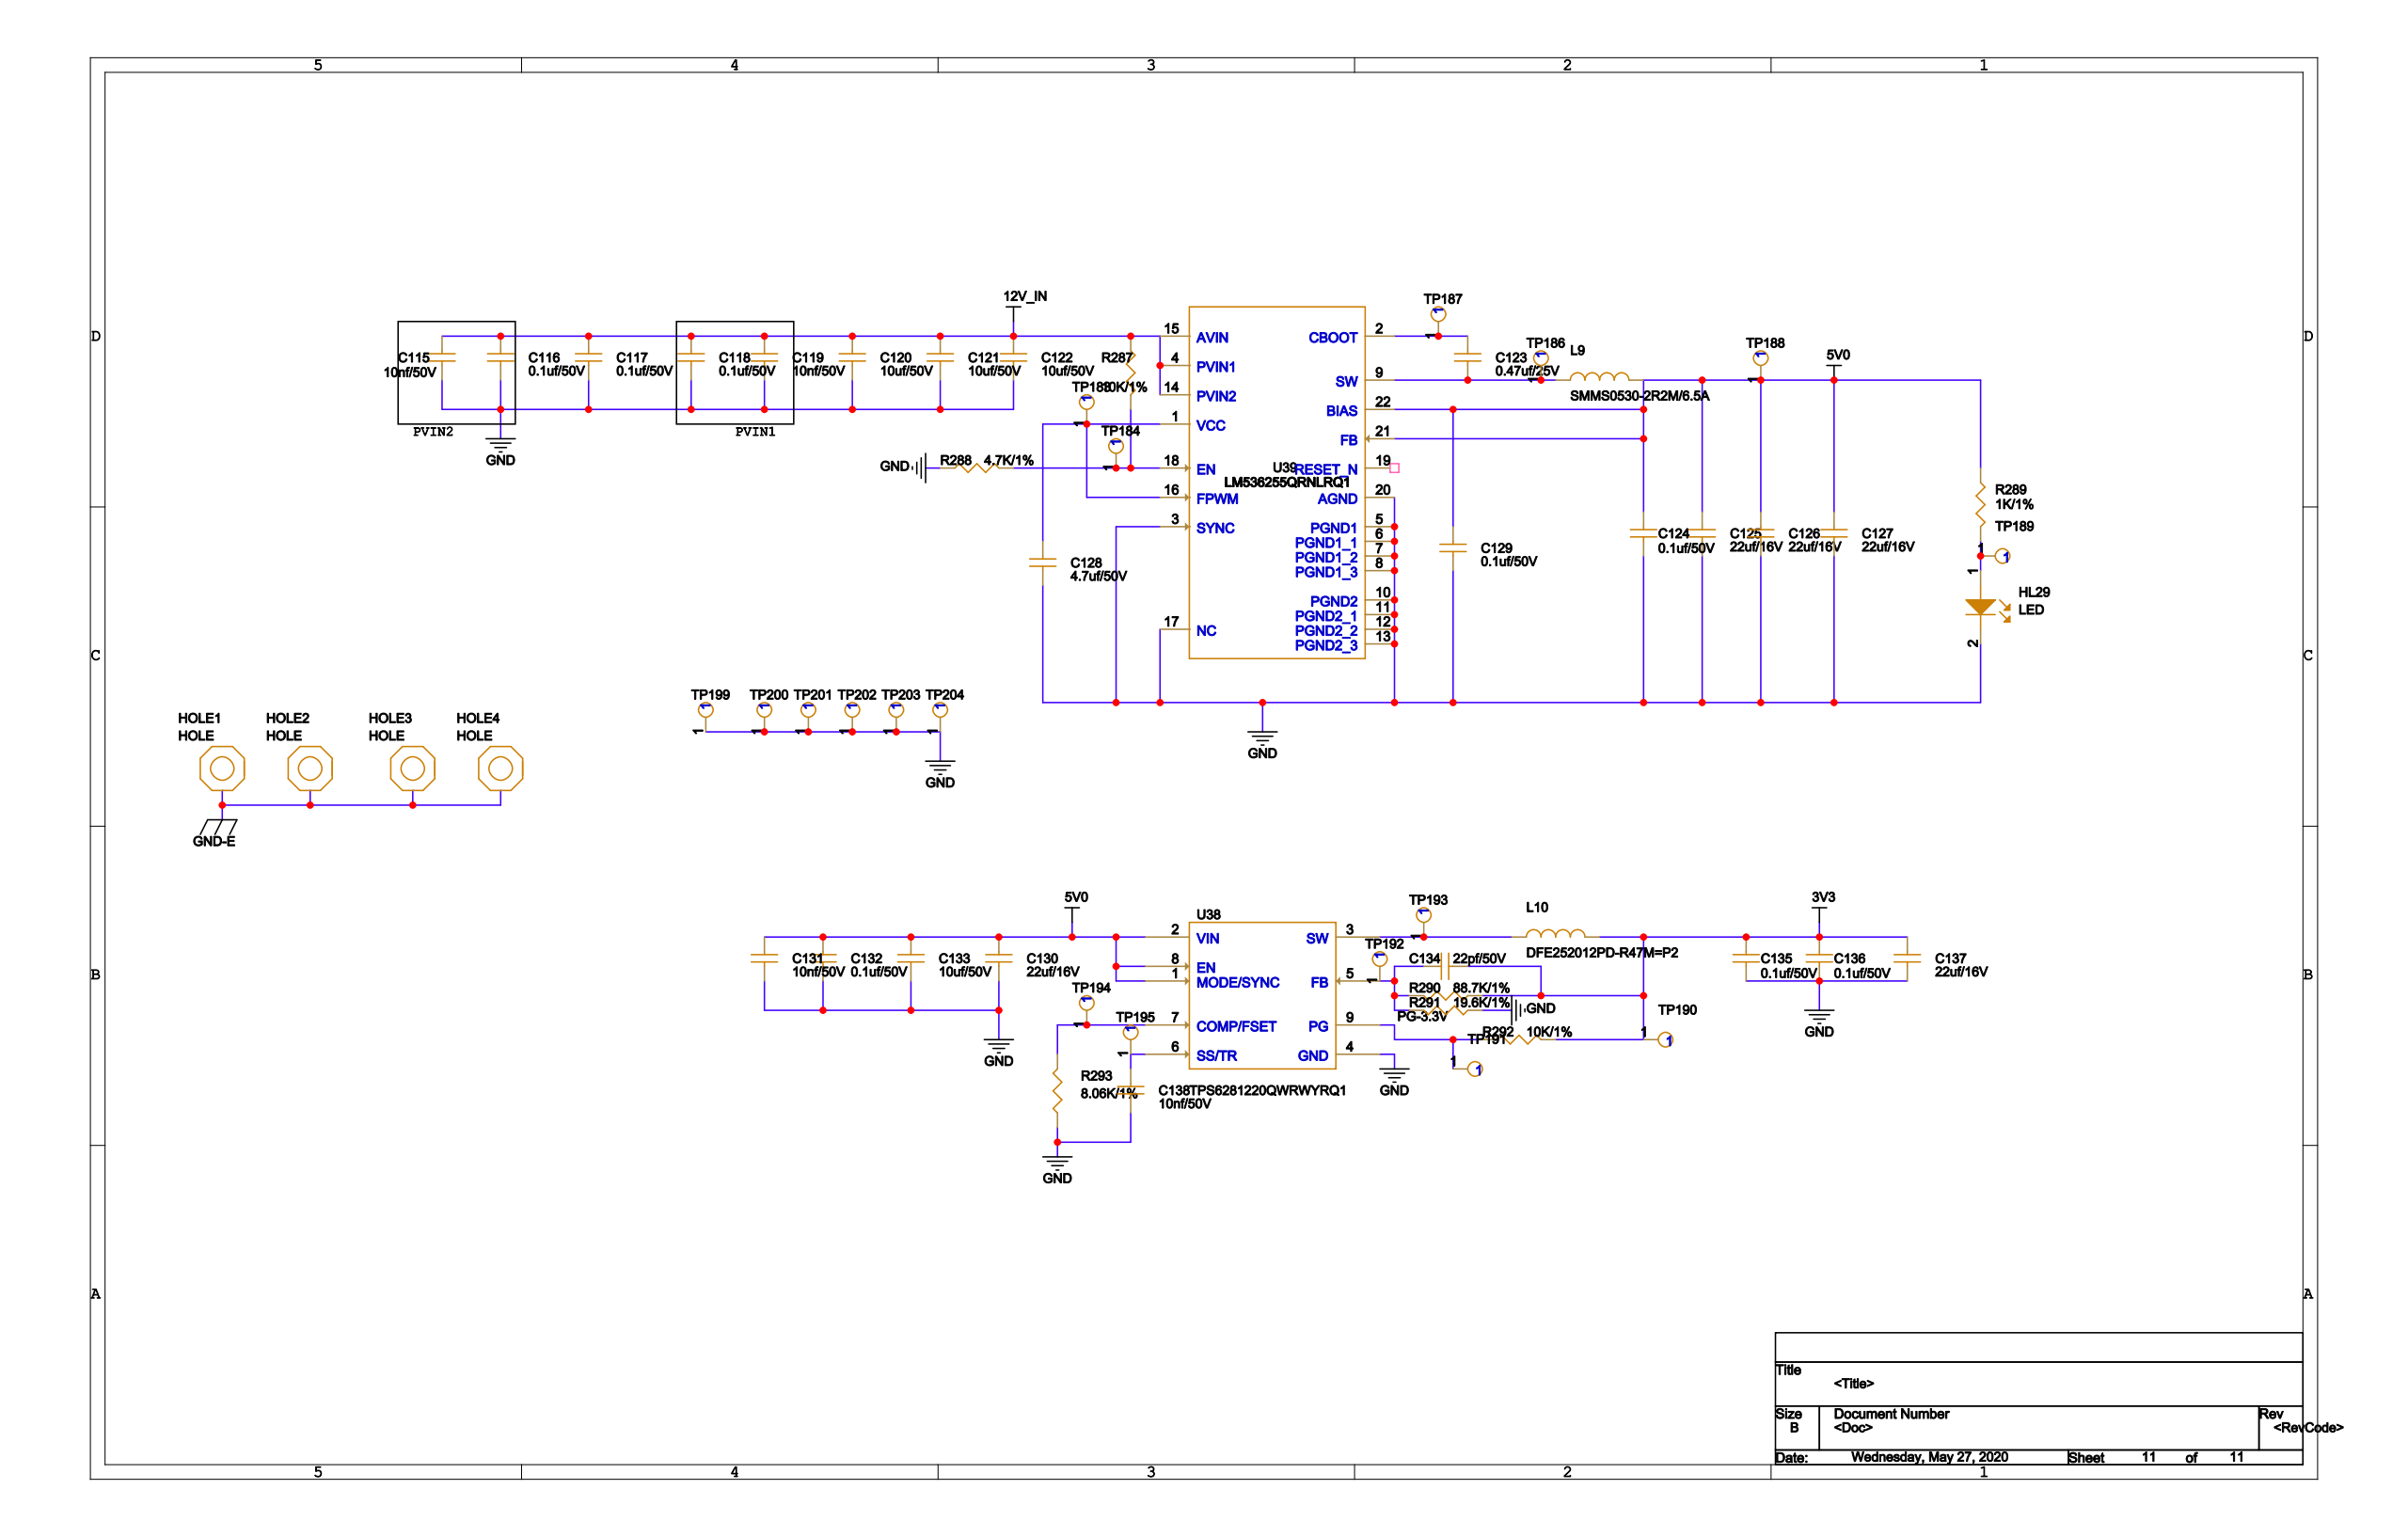Circuit board | Cadence Allegro | 521 parts | 239 nets | one sheet of the schematic
Parts on this sheet (reference | value | footprint):
C115 | 10nf/50V | C0402
C116 | 0.1uf/50V | C0402
C117 | 0.1uf/50V | C0402
C118 | 0.1uf/50V | C0402
C119 | 10nf/50V | C0402
C120 | 10uf/50V | C0805
C121 | 10uf/50V | C0805
C122 | 10uf/50V | C0805
C123 | 0.47uf/25V | C0402
C124 | 0.1uf/50V | C0402
C125 | 22uf/16V | C1210
C126 | 22uf/16V | C1210
C127 | 22uf/16V | C1210
C128 | 4.7uf/50V | C0805
C129 | 0.1uf/50V | C0402
C130 | 22uf/16V | C1210
C131 | 10nf/50V | C0402
C132 | 0.1uf/50V | C0402
C133 | 10uf/50V | C0805
C134 | 22pf/50V | C0402
C135 | 0.1uf/50V | C0402
C136 | 0.1uf/50V | C0402
C137 | 22uf/16V | C1210
C138 | 10nf/50V | C0402
HL29 | LED | LED0603
HOLE1 | HOLE | HOLEPAD_50X30
HOLE2 | HOLE | HOLEPAD_50X30
HOLE3 | HOLE | HOLEPAD_50X30
HOLE4 | HOLE | HOLEPAD_50X30
L9 | SMMS0530-2R2M/6.5A | SM_IND_5L
L10 | DFE252012PD-R47M=P2 | SM_IND_3L
R287 | 10K/1% | 0402
R288 | 4.7K/1% | 0402
R289 | 1K/1% | R0603
R290 | 88.7K/1% | 0603
R291 | 19.6K/1% | 0603
R292 | 10K/1% | 0603
R293 | 8.06K/1% | 0402
TP183 | TESTPOINT | TESTPOINT-33MIL
TP184 | TESTPOINT | TESTPOINT-33MIL
TP186 | TESTPOINT | TESTPOINT-33MIL
TP187 | TESTPOINT | TESTPOINT-33MIL
TP188 | TESTPOINT | TESTPOINT-33MIL
TP189 | TESTPOINT | TESTPOINT-33MIL
TP190 | TESTPOINT | TESTPOINT-33MIL
TP191 | TESTPOINT | TESTPOINT-33MIL
TP192 | TESTPOINT | TESTPOINT-33MIL
TP193 | TESTPOINT | TESTPOINT-33MIL
TP194 | TESTPOINT | TESTPOINT-33MIL
TP195 | TESTPOINT | TESTPOINT-33MIL
TP199 | TESTPOINT | TESTPOINT-33MIL
TP200 | TESTPOINT | TESTPOINT-33MIL
TP201 | TESTPOINT | TESTPOINT-33MIL
TP202 | TESTPOINT | TESTPOINT-33MIL
TP203 | TESTPOINT | TESTPOINT-33MIL
TP204 | TESTPOINT | TESTPOINT-33MIL
U38 | TPS6281220QWRWYRQ1 | RWY0009A
U39 | LM536255QRNLRQ1 | RNL0022A_NV
Nets of these parts (net: part-pin ...):
GND: C115-2 C116-2 C117-2 C118-2 C119-2 C120-2 C121-2 C122-2 C124-2 C125-2 C126-2 C127-2 C128-2 C129-2 C130-2 C131-2 C132-2 C133-2 C135-2 C136-2 C137-2 C138-2 HL29-2 R288-1 R291-1 R293-1 TP199-1 TP200-1 TP201-1 TP202-1 TP203-1 TP204-1 U38-4 U39-3 U39-5 U39-6 U39-7 U39-8 U39-10 U39-11 U39-12 U39-13 U39-17 U39-20
12V_IN: C115-1 C116-1 C117-1 C118-1 C119-1 C120-1 C121-1 C122-1 R287-1 U39-4 U39-14 U39-15
N7539499: L10-1 TP193-1 U38-3
3V3: C134-2 C135-1 C136-1 C137-1 L10-2 R290-1 R292-2 TP190-1
PG-3.3V: R292-1 TP191-1 U38-9
N7538390: R293-2 TP194-1 U38-7
GND-E: HOLE1-1 HOLE2-1 HOLE3-1 HOLE4-1
N7278733: C128-1 TP183-1 U39-1 U39-16
N7278425: R287-2 R288-2 TP184-1 U39-18
N7278841: C123-2 L9-1 TP186-1 U39-9
N7278865: C123-1 TP187-1 U39-2
5V0: C124-1 C125-1 C126-1 C127-1 C129-1 C130-1 C131-1 C132-1 C133-1 L9-2 R289-1 TP188-1 U38-1 U38-2 U38-8 U39-21 U39-22
N7845429: HL29-1 R289-2 TP189-1
N7539563: C134-1 R290-2 R291-2 TP192-1 U38-5
N7538521: C138-1 TP195-1 U38-6